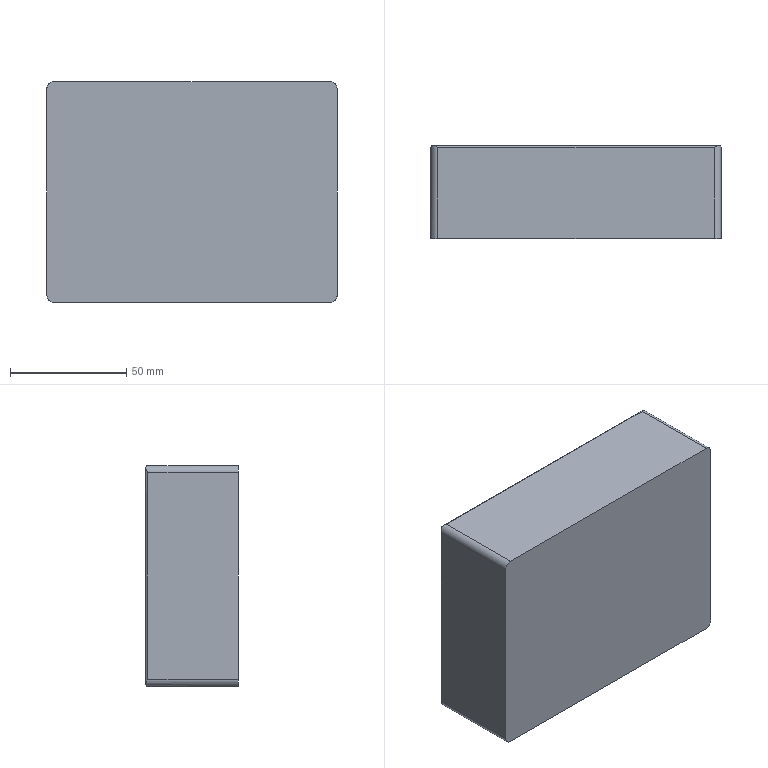Part | SolidWorks | features BaseBody 1 | 1 solid | 20 faces | box 125 x 40 x 95 mm | volume 474597 mm3 | cylinder 8 | cone 6 | plane 6 | commonest cylinder face diameters 2 x4 6 x4
STEP:
#1=CARTESIAN_POINT('',(353.,-93.,-55.087));
#2=VERTEX_POINT('',#1);
#3=CARTESIAN_POINT('',(353.,-92.,-56.087));
#4=VERTEX_POINT('',#3);
#5=CARTESIAN_POINT('',(353.,-92.,-56.087));
#6=DIRECTION('',(0.,0.7071,-0.7071));
#7=VECTOR('',#6,1000.);
#8=LINE('',#5,#7);
#9=EDGE_CURVE('',#2,#4,#8,.T.);
#10=ORIENTED_EDGE('',*,*,#9,.F.);
#11=CARTESIAN_POINT('',(353.,-94.,-56.087));
#12=VERTEX_POINT('',#11);
#13=CARTESIAN_POINT('',(353.,-94.,-56.087));
#14=DIRECTION('',(0.,-0.7071,-0.7071));
#15=VECTOR('',#14,1000.);
#16=LINE('',#13,#15);
#17=EDGE_CURVE('',#2,#12,#16,.T.);
#18=ORIENTED_EDGE('',*,*,#17,.T.);
#19=CARTESIAN_POINT('',(353.,-93.,-56.087));
#20=DIRECTION('',(0.,0.,1.));
#21=DIRECTION('',(0.,1.,0.));
#22=AXIS2_PLACEMENT_3D('',#19,#20,#21);
#23=CIRCLE('',#22,1.);
#24=EDGE_CURVE('',#4,#12,#23,.T.);
#25=ORIENTED_EDGE('',*,*,#24,.F.);
#26=EDGE_LOOP('',(#10,#18,#25));
#27=FACE_OUTER_BOUND('',#26,.T.);
#28=CARTESIAN_POINT('',(353.,-93.,-56.087));
#29=DIRECTION('',(0.,0.,-1.));
#30=DIRECTION('',(0.,1.,0.));
#31=AXIS2_PLACEMENT_3D('',#28,#29,#30);
#32=CONICAL_SURFACE('',#31,1.,0.7854);
#33=ADVANCED_FACE('',(#27),#32,.F.);
#34=CARTESIAN_POINT('',(284.,-93.,-55.087));
#35=VERTEX_POINT('',#34);
#36=CARTESIAN_POINT('',(283.,-93.,-56.087));
#37=VERTEX_POINT('',#36);
#38=CARTESIAN_POINT('',(283.,-93.,-56.087));
#39=DIRECTION('',(-0.7071,0.,-0.7071));
#40=VECTOR('',#39,1000.);
#41=LINE('',#38,#40);
#42=EDGE_CURVE('',#35,#37,#41,.T.);
#43=ORIENTED_EDGE('',*,*,#42,.F.);
#44=CARTESIAN_POINT('',(285.,-93.,-56.087));
#45=VERTEX_POINT('',#44);
#46=CARTESIAN_POINT('',(285.,-93.,-56.087));
#47=DIRECTION('',(0.7071,0.,-0.7071));
#48=VECTOR('',#47,1000.);
#49=LINE('',#46,#48);
#50=EDGE_CURVE('',#35,#45,#49,.T.);
#51=ORIENTED_EDGE('',*,*,#50,.T.);
#52=CARTESIAN_POINT('',(284.,-93.,-56.087));
#53=DIRECTION('',(0.,0.,1.));
#54=DIRECTION('',(-1.,0.,0.));
#55=AXIS2_PLACEMENT_3D('',#52,#53,#54);
#56=CIRCLE('',#55,1.);
#57=EDGE_CURVE('',#37,#45,#56,.T.);
#58=ORIENTED_EDGE('',*,*,#57,.F.);
#59=EDGE_LOOP('',(#43,#51,#58));
#60=FACE_OUTER_BOUND('',#59,.T.);
#61=CARTESIAN_POINT('',(284.,-93.,-56.087));
#62=DIRECTION('',(0.,0.,-1.));
#63=DIRECTION('',(-1.,0.,0.));
#64=AXIS2_PLACEMENT_3D('',#61,#62,#63);
#65=CONICAL_SURFACE('',#64,1.,0.7854);
#66=ADVANCED_FACE('',(#60),#65,.F.);
#67=CARTESIAN_POINT('',(320.,-93.,-55.087));
#68=VERTEX_POINT('',#67);
#69=CARTESIAN_POINT('',(319.,-93.,-56.087));
#70=VERTEX_POINT('',#69);
#71=CARTESIAN_POINT('',(319.,-93.,-56.087));
#72=DIRECTION('',(-0.7071,0.,-0.7071));
#73=VECTOR('',#72,1000.);
#74=LINE('',#71,#73);
#75=EDGE_CURVE('',#68,#70,#74,.T.);
#76=ORIENTED_EDGE('',*,*,#75,.F.);
#77=CARTESIAN_POINT('',(321.,-93.,-56.087));
#78=VERTEX_POINT('',#77);
#79=CARTESIAN_POINT('',(321.,-93.,-56.087));
#80=DIRECTION('',(0.7071,0.,-0.7071));
#81=VECTOR('',#80,1000.);
#82=LINE('',#79,#81);
#83=EDGE_CURVE('',#68,#78,#82,.T.);
#84=ORIENTED_EDGE('',*,*,#83,.T.);
#85=CARTESIAN_POINT('',(320.,-93.,-56.087));
#86=DIRECTION('',(0.,0.,1.));
#87=DIRECTION('',(-1.,0.,0.));
#88=AXIS2_PLACEMENT_3D('',#85,#86,#87);
#89=CIRCLE('',#88,1.);
#90=EDGE_CURVE('',#70,#78,#89,.T.);
#91=ORIENTED_EDGE('',*,*,#90,.F.);
#92=EDGE_LOOP('',(#76,#84,#91));
#93=FACE_OUTER_BOUND('',#92,.T.);
#94=CARTESIAN_POINT('',(320.,-93.,-56.087));
#95=DIRECTION('',(0.,0.,-1.));
#96=DIRECTION('',(-1.,0.,0.));
#97=AXIS2_PLACEMENT_3D('',#94,#95,#96);
#98=CONICAL_SURFACE('',#97,1.,0.7854);
#99=ADVANCED_FACE('',(#93),#98,.F.);
#100=CARTESIAN_POINT('',(381.5,-114.,38.913));
#101=VERTEX_POINT('',#100);
#102=CARTESIAN_POINT('',(262.5,-114.,38.913));
#103=VERTEX_POINT('',#102);
#104=CARTESIAN_POINT('',(322.,-114.,38.913));
#105=DIRECTION('',(-1.,0.,0.));
#106=VECTOR('',#105,1000.);
#107=LINE('',#104,#106);
#108=EDGE_CURVE('',#101,#103,#107,.T.);
#109=ORIENTED_EDGE('',*,*,#108,.T.);
#110=CARTESIAN_POINT('',(259.5,-114.,35.913));
#111=VERTEX_POINT('',#110);
#112=CARTESIAN_POINT('',(262.5,-114.,35.913));
#113=DIRECTION('',(0.,-1.,0.));
#114=DIRECTION('',(0.,0.,-1.));
#115=AXIS2_PLACEMENT_3D('',#112,#113,#114);
#116=CIRCLE('',#115,3.);
#117=EDGE_CURVE('',#103,#111,#116,.T.);
#118=ORIENTED_EDGE('',*,*,#117,.T.);
#119=CARTESIAN_POINT('',(259.5,-114.,-53.087));
#120=VERTEX_POINT('',#119);
#121=CARTESIAN_POINT('',(259.5,-114.,-8.587));
#122=DIRECTION('',(0.,0.,-1.));
#123=VECTOR('',#122,1000.);
#124=LINE('',#121,#123);
#125=EDGE_CURVE('',#111,#120,#124,.T.);
#126=ORIENTED_EDGE('',*,*,#125,.T.);
#127=CARTESIAN_POINT('',(262.5,-114.,-56.087));
#128=VERTEX_POINT('',#127);
#129=CARTESIAN_POINT('',(262.5,-114.,-53.087));
#130=DIRECTION('',(0.,-1.,0.));
#131=DIRECTION('',(0.,0.,-1.));
#132=AXIS2_PLACEMENT_3D('',#129,#130,#131);
#133=CIRCLE('',#132,3.);
#134=EDGE_CURVE('',#120,#128,#133,.T.);
#135=ORIENTED_EDGE('',*,*,#134,.T.);
#136=CARTESIAN_POINT('',(381.5,-114.,-56.087));
#137=VERTEX_POINT('',#136);
#138=CARTESIAN_POINT('',(322.,-114.,-56.087));
#139=DIRECTION('',(1.,0.,0.));
#140=VECTOR('',#139,1000.);
#141=LINE('',#138,#140);
#142=EDGE_CURVE('',#128,#137,#141,.T.);
#143=ORIENTED_EDGE('',*,*,#142,.T.);
#144=CARTESIAN_POINT('',(384.5,-114.,-53.087));
#145=VERTEX_POINT('',#144);
#146=CARTESIAN_POINT('',(381.5,-114.,-53.087));
#147=DIRECTION('',(0.,-1.,0.));
#148=DIRECTION('',(0.,0.,-1.));
#149=AXIS2_PLACEMENT_3D('',#146,#147,#148);
#150=CIRCLE('',#149,3.);
#151=EDGE_CURVE('',#137,#145,#150,.T.);
#152=ORIENTED_EDGE('',*,*,#151,.T.);
#153=CARTESIAN_POINT('',(384.5,-114.,35.913));
#154=VERTEX_POINT('',#153);
#155=CARTESIAN_POINT('',(384.5,-114.,-8.587));
#156=DIRECTION('',(0.,0.,1.));
#157=VECTOR('',#156,1000.);
#158=LINE('',#155,#157);
#159=EDGE_CURVE('',#145,#154,#158,.T.);
#160=ORIENTED_EDGE('',*,*,#159,.T.);
#161=CARTESIAN_POINT('',(381.5,-114.,35.913));
#162=DIRECTION('',(0.,-1.,0.));
#163=DIRECTION('',(0.,0.,-1.));
#164=AXIS2_PLACEMENT_3D('',#161,#162,#163);
#165=CIRCLE('',#164,3.);
#166=EDGE_CURVE('',#154,#101,#165,.T.);
#167=ORIENTED_EDGE('',*,*,#166,.T.);
#168=EDGE_LOOP('',(#109,#118,#126,#135,#143,#152,#160,#167));
#169=FACE_OUTER_BOUND('',#168,.T.);
#170=CARTESIAN_POINT('',(322.,-114.,-8.587));
#171=DIRECTION('',(0.,-1.,0.));
#172=DIRECTION('',(0.,0.,-1.));
#173=AXIS2_PLACEMENT_3D('',#170,#171,#172);
#174=PLANE('',#173);
#175=ADVANCED_FACE('',(#169),#174,.T.);
#176=CARTESIAN_POINT('',(262.5,-75.,38.913));
#177=VERTEX_POINT('',#176);
#178=CARTESIAN_POINT('',(262.5,-74.,38.913));
#179=DIRECTION('',(0.,1.,0.));
#180=VECTOR('',#179,1000.);
#181=LINE('',#178,#180);
#182=EDGE_CURVE('',#103,#177,#181,.T.);
#183=ORIENTED_EDGE('',*,*,#182,.T.);
#184=CARTESIAN_POINT('',(260.379,-74.007,38.034));
#185=VERTEX_POINT('',#184);
#186=CARTESIAN_POINT('',(262.5,-75.,38.913));
#187=CARTESIAN_POINT('',(262.408,-74.947,38.913));
#188=CARTESIAN_POINT('',(262.314,-74.892,38.909));
#189=CARTESIAN_POINT('',(262.129,-74.786,38.891));
#190=CARTESIAN_POINT('',(262.037,-74.734,38.878));
#191=CARTESIAN_POINT('',(261.762,-74.579,38.827));
#192=CARTESIAN_POINT('',(261.58,-74.48,38.775));
#193=CARTESIAN_POINT('',(261.216,-74.295,38.631));
#194=CARTESIAN_POINT('',(261.039,-74.211,38.541));
#195=CARTESIAN_POINT('',(260.697,-74.077,38.319));
#196=CARTESIAN_POINT('',(260.531,-74.026,38.186));
#197=CARTESIAN_POINT('',(260.379,-74.007,38.034));
#198=B_SPLINE_CURVE_WITH_KNOTS('',3,(#186,#187,#188,#189,#190,#191,#192,#193,#194,#195,#196,#197),.UNSPECIFIED.,.F.,.F.,(4,2,2,2,2,4),(-0.00001095,0.0003086,0.0006282,0.001267,0.001907,0.002546),.UNSPECIFIED.);
#199=EDGE_CURVE('',#177,#185,#198,.T.);
#200=ORIENTED_EDGE('',*,*,#199,.T.);
#201=CARTESIAN_POINT('',(259.5,-75.,35.913));
#202=VERTEX_POINT('',#201);
#203=CARTESIAN_POINT('',(260.379,-74.007,38.034));
#204=CARTESIAN_POINT('',(260.226,-74.026,37.881));
#205=CARTESIAN_POINT('',(260.096,-74.076,37.719));
#206=CARTESIAN_POINT('',(259.872,-74.211,37.374));
#207=CARTESIAN_POINT('',(259.782,-74.294,37.198));
#208=CARTESIAN_POINT('',(259.569,-74.568,36.659));
#209=CARTESIAN_POINT('',(259.5,-74.786,36.284));
#210=CARTESIAN_POINT('',(259.5,-75.,35.913));
#211=B_SPLINE_CURVE_WITH_KNOTS('',3,(#203,#204,#205,#206,#207,#208,#209,#210),.UNSPECIFIED.,.F.,.F.,(4,2,2,4),(0.,0.0006423,0.001285,0.002569),.UNSPECIFIED.);
#212=EDGE_CURVE('',#185,#202,#211,.T.);
#213=ORIENTED_EDGE('',*,*,#212,.T.);
#214=CARTESIAN_POINT('',(259.5,-74.,35.913));
#215=DIRECTION('',(0.,-1.,0.));
#216=VECTOR('',#215,1000.);
#217=LINE('',#214,#216);
#218=EDGE_CURVE('',#202,#111,#217,.T.);
#219=ORIENTED_EDGE('',*,*,#218,.T.);
#220=ORIENTED_EDGE('',*,*,#117,.F.);
#221=EDGE_LOOP('',(#183,#200,#213,#219,#220));
#222=FACE_OUTER_BOUND('',#221,.T.);
#223=CARTESIAN_POINT('',(262.5,-74.,35.913));
#224=DIRECTION('',(0.,-1.,0.));
#225=DIRECTION('',(0.,0.,-1.));
#226=AXIS2_PLACEMENT_3D('',#223,#224,#225);
#227=CYLINDRICAL_SURFACE('',#226,3.);
#228=ADVANCED_FACE('',(#222),#227,.T.);
#229=CARTESIAN_POINT('',(381.5,-75.,38.913));
#230=VERTEX_POINT('',#229);
#231=CARTESIAN_POINT('',(262.5,-75.,38.913));
#232=DIRECTION('',(-1.,0.,0.));
#233=VECTOR('',#232,1000.);
#234=LINE('',#231,#233);
#235=EDGE_CURVE('',#230,#177,#234,.T.);
#236=ORIENTED_EDGE('',*,*,#235,.T.);
#237=ORIENTED_EDGE('',*,*,#182,.F.);
#238=ORIENTED_EDGE('',*,*,#108,.F.);
#239=CARTESIAN_POINT('',(381.5,-74.,38.913));
#240=DIRECTION('',(0.,1.,0.));
#241=VECTOR('',#240,1000.);
#242=LINE('',#239,#241);
#243=EDGE_CURVE('',#101,#230,#242,.T.);
#244=ORIENTED_EDGE('',*,*,#243,.T.);
#245=EDGE_LOOP('',(#236,#237,#238,#244));
#246=FACE_OUTER_BOUND('',#245,.T.);
#247=CARTESIAN_POINT('',(262.5,-74.,38.913));
#248=DIRECTION('',(0.,0.,1.));
#249=DIRECTION('',(1.,0.,0.));
#250=AXIS2_PLACEMENT_3D('',#247,#248,#249);
#251=PLANE('',#250);
#252=ADVANCED_FACE('',(#246),#251,.T.);
#253=CARTESIAN_POINT('',(384.5,-75.,35.913));
#254=VERTEX_POINT('',#253);
#255=CARTESIAN_POINT('',(383.621,-74.007,38.034));
#256=VERTEX_POINT('',#255);
#257=CARTESIAN_POINT('',(384.5,-75.,35.913));
#258=CARTESIAN_POINT('',(384.5,-74.947,36.005));
#259=CARTESIAN_POINT('',(384.496,-74.892,36.099));
#260=CARTESIAN_POINT('',(384.478,-74.786,36.284));
#261=CARTESIAN_POINT('',(384.465,-74.734,36.376));
#262=CARTESIAN_POINT('',(384.414,-74.579,36.651));
#263=CARTESIAN_POINT('',(384.362,-74.48,36.833));
#264=CARTESIAN_POINT('',(384.218,-74.295,37.197));
#265=CARTESIAN_POINT('',(384.128,-74.211,37.374));
#266=CARTESIAN_POINT('',(383.906,-74.077,37.716));
#267=CARTESIAN_POINT('',(383.773,-74.026,37.882));
#268=CARTESIAN_POINT('',(383.621,-74.007,38.034));
#269=B_SPLINE_CURVE_WITH_KNOTS('',3,(#257,#258,#259,#260,#261,#262,#263,#264,#265,#266,#267,#268),.UNSPECIFIED.,.F.,.F.,(4,2,2,2,2,4),(-0.00001095,0.0003086,0.0006282,0.001267,0.001907,0.002546),.UNSPECIFIED.);
#270=EDGE_CURVE('',#254,#256,#269,.T.);
#271=ORIENTED_EDGE('',*,*,#270,.T.);
#272=CARTESIAN_POINT('',(383.621,-74.007,38.034));
#273=CARTESIAN_POINT('',(383.468,-74.026,38.187));
#274=CARTESIAN_POINT('',(383.306,-74.076,38.317));
#275=CARTESIAN_POINT('',(382.961,-74.211,38.541));
#276=CARTESIAN_POINT('',(382.785,-74.294,38.631));
#277=CARTESIAN_POINT('',(382.246,-74.568,38.844));
#278=CARTESIAN_POINT('',(381.871,-74.786,38.913));
#279=CARTESIAN_POINT('',(381.5,-75.,38.913));
#280=B_SPLINE_CURVE_WITH_KNOTS('',3,(#272,#273,#274,#275,#276,#277,#278,#279),.UNSPECIFIED.,.F.,.F.,(4,2,2,4),(0.,0.0006423,0.001285,0.002569),.UNSPECIFIED.);
#281=EDGE_CURVE('',#256,#230,#280,.T.);
#282=ORIENTED_EDGE('',*,*,#281,.T.);
#283=ORIENTED_EDGE('',*,*,#243,.F.);
#284=ORIENTED_EDGE('',*,*,#166,.F.);
#285=CARTESIAN_POINT('',(384.5,-74.,35.913));
#286=DIRECTION('',(0.,1.,0.));
#287=VECTOR('',#286,1000.);
#288=LINE('',#285,#287);
#289=EDGE_CURVE('',#154,#254,#288,.T.);
#290=ORIENTED_EDGE('',*,*,#289,.T.);
#291=EDGE_LOOP('',(#271,#282,#283,#284,#290));
#292=FACE_OUTER_BOUND('',#291,.T.);
#293=CARTESIAN_POINT('',(381.5,-74.,35.913));
#294=DIRECTION('',(0.,-1.,0.));
#295=DIRECTION('',(0.,0.,-1.));
#296=AXIS2_PLACEMENT_3D('',#293,#294,#295);
#297=CYLINDRICAL_SURFACE('',#296,3.);
#298=ADVANCED_FACE('',(#292),#297,.T.);
#299=CARTESIAN_POINT('',(384.5,-75.,-53.087));
#300=VERTEX_POINT('',#299);
#301=CARTESIAN_POINT('',(384.5,-75.,35.913));
#302=DIRECTION('',(0.,0.,1.));
#303=VECTOR('',#302,1000.);
#304=LINE('',#301,#303);
#305=EDGE_CURVE('',#300,#254,#304,.T.);
#306=ORIENTED_EDGE('',*,*,#305,.T.);
#307=ORIENTED_EDGE('',*,*,#289,.F.);
#308=ORIENTED_EDGE('',*,*,#159,.F.);
#309=CARTESIAN_POINT('',(384.5,-74.,-53.087));
#310=DIRECTION('',(0.,1.,0.));
#311=VECTOR('',#310,1000.);
#312=LINE('',#309,#311);
#313=EDGE_CURVE('',#145,#300,#312,.T.);
#314=ORIENTED_EDGE('',*,*,#313,.T.);
#315=EDGE_LOOP('',(#306,#307,#308,#314));
#316=FACE_OUTER_BOUND('',#315,.T.);
#317=CARTESIAN_POINT('',(384.5,-74.,35.913));
#318=DIRECTION('',(1.,0.,0.));
#319=DIRECTION('',(0.,0.,-1.));
#320=AXIS2_PLACEMENT_3D('',#317,#318,#319);
#321=PLANE('',#320);
#322=ADVANCED_FACE('',(#316),#321,.T.);
#323=CARTESIAN_POINT('',(381.5,-75.,-56.087));
#324=VERTEX_POINT('',#323);
#325=CARTESIAN_POINT('',(381.5,-74.,-56.087));
#326=DIRECTION('',(0.,1.,0.));
#327=VECTOR('',#326,1000.);
#328=LINE('',#325,#327);
#329=EDGE_CURVE('',#137,#324,#328,.T.);
#330=ORIENTED_EDGE('',*,*,#329,.T.);
#331=CARTESIAN_POINT('',(383.621,-74.007,-55.208));
#332=VERTEX_POINT('',#331);
#333=CARTESIAN_POINT('',(381.5,-75.,-56.087));
#334=CARTESIAN_POINT('',(381.592,-74.947,-56.087));
#335=CARTESIAN_POINT('',(381.686,-74.892,-56.083));
#336=CARTESIAN_POINT('',(381.871,-74.786,-56.065));
#337=CARTESIAN_POINT('',(381.963,-74.734,-56.052));
#338=CARTESIAN_POINT('',(382.238,-74.579,-56.001));
#339=CARTESIAN_POINT('',(382.42,-74.48,-55.949));
#340=CARTESIAN_POINT('',(382.784,-74.295,-55.805));
#341=CARTESIAN_POINT('',(382.961,-74.211,-55.715));
#342=CARTESIAN_POINT('',(383.303,-74.077,-55.493));
#343=CARTESIAN_POINT('',(383.469,-74.026,-55.36));
#344=CARTESIAN_POINT('',(383.621,-74.007,-55.208));
#345=B_SPLINE_CURVE_WITH_KNOTS('',3,(#333,#334,#335,#336,#337,#338,#339,#340,#341,#342,#343,#344),.UNSPECIFIED.,.F.,.F.,(4,2,2,2,2,4),(-0.00001095,0.0003086,0.0006282,0.001267,0.001907,0.002546),.UNSPECIFIED.);
#346=EDGE_CURVE('',#324,#332,#345,.T.);
#347=ORIENTED_EDGE('',*,*,#346,.T.);
#348=CARTESIAN_POINT('',(383.621,-74.007,-55.208));
#349=CARTESIAN_POINT('',(383.774,-74.026,-55.055));
#350=CARTESIAN_POINT('',(383.904,-74.076,-54.893));
#351=CARTESIAN_POINT('',(384.128,-74.211,-54.548));
#352=CARTESIAN_POINT('',(384.218,-74.294,-54.372));
#353=CARTESIAN_POINT('',(384.431,-74.568,-53.833));
#354=CARTESIAN_POINT('',(384.5,-74.786,-53.458));
#355=CARTESIAN_POINT('',(384.5,-75.,-53.087));
#356=B_SPLINE_CURVE_WITH_KNOTS('',3,(#348,#349,#350,#351,#352,#353,#354,#355),.UNSPECIFIED.,.F.,.F.,(4,2,2,4),(0.,0.0006423,0.001285,0.002569),.UNSPECIFIED.);
#357=EDGE_CURVE('',#332,#300,#356,.T.);
#358=ORIENTED_EDGE('',*,*,#357,.T.);
#359=ORIENTED_EDGE('',*,*,#313,.F.);
#360=ORIENTED_EDGE('',*,*,#151,.F.);
#361=EDGE_LOOP('',(#330,#347,#358,#359,#360));
#362=FACE_OUTER_BOUND('',#361,.T.);
#363=CARTESIAN_POINT('',(381.5,-74.,-53.087));
#364=DIRECTION('',(0.,-1.,0.));
#365=DIRECTION('',(0.,0.,-1.));
#366=AXIS2_PLACEMENT_3D('',#363,#364,#365);
#367=CYLINDRICAL_SURFACE('',#366,3.);
#368=ADVANCED_FACE('',(#362),#367,.T.);
#369=ORIENTED_EDGE('',*,*,#24,.T.);
#370=CARTESIAN_POINT('',(353.,-93.,-56.087));
#371=DIRECTION('',(0.,0.,1.));
#372=DIRECTION('',(0.,1.,0.));
#373=AXIS2_PLACEMENT_3D('',#370,#371,#372);
#374=CIRCLE('',#373,1.);
#375=EDGE_CURVE('',#12,#4,#374,.T.);
#376=ORIENTED_EDGE('',*,*,#375,.T.);
#377=EDGE_LOOP('',(#369,#376));
#378=FACE_BOUND('',#377,.T.);
#379=ORIENTED_EDGE('',*,*,#57,.T.);
#380=CARTESIAN_POINT('',(284.,-93.,-56.087));
#381=DIRECTION('',(0.,0.,1.));
#382=DIRECTION('',(-1.,0.,0.));
#383=AXIS2_PLACEMENT_3D('',#380,#381,#382);
#384=CIRCLE('',#383,1.);
#385=EDGE_CURVE('',#45,#37,#384,.T.);
#386=ORIENTED_EDGE('',*,*,#385,.T.);
#387=EDGE_LOOP('',(#379,#386));
#388=FACE_BOUND('',#387,.T.);
#389=ORIENTED_EDGE('',*,*,#90,.T.);
#390=CARTESIAN_POINT('',(320.,-93.,-56.087));
#391=DIRECTION('',(0.,0.,1.));
#392=DIRECTION('',(-1.,0.,0.));
#393=AXIS2_PLACEMENT_3D('',#390,#391,#392);
#394=CIRCLE('',#393,1.);
#395=EDGE_CURVE('',#78,#70,#394,.T.);
#396=ORIENTED_EDGE('',*,*,#395,.T.);
#397=EDGE_LOOP('',(#389,#396));
#398=FACE_BOUND('',#397,.T.);
#399=CARTESIAN_POINT('',(262.5,-75.,-56.087));
#400=VERTEX_POINT('',#399);
#401=CARTESIAN_POINT('',(381.5,-75.,-56.087));
#402=DIRECTION('',(1.,0.,0.));
#403=VECTOR('',#402,1000.);
#404=LINE('',#401,#403);
#405=EDGE_CURVE('',#400,#324,#404,.T.);
#406=ORIENTED_EDGE('',*,*,#405,.T.);
#407=ORIENTED_EDGE('',*,*,#329,.F.);
#408=ORIENTED_EDGE('',*,*,#142,.F.);
#409=CARTESIAN_POINT('',(262.5,-74.,-56.087));
#410=DIRECTION('',(0.,1.,0.));
#411=VECTOR('',#410,1000.);
#412=LINE('',#409,#411);
#413=EDGE_CURVE('',#128,#400,#412,.T.);
#414=ORIENTED_EDGE('',*,*,#413,.T.);
#415=EDGE_LOOP('',(#406,#407,#408,#414));
#416=FACE_OUTER_BOUND('',#415,.T.);
#417=CARTESIAN_POINT('',(381.5,-74.,-56.087));
#418=DIRECTION('',(0.,0.,-1.));
#419=DIRECTION('',(-1.,0.,0.));
#420=AXIS2_PLACEMENT_3D('',#417,#418,#419);
#421=PLANE('',#420);
#422=ADVANCED_FACE('',(#378,#388,#398,#416),#421,.T.);
#423=CARTESIAN_POINT('',(259.5,-75.,-53.087));
#424=VERTEX_POINT('',#423);
#425=CARTESIAN_POINT('',(260.379,-74.007,-55.208));
#426=VERTEX_POINT('',#425);
#427=CARTESIAN_POINT('',(259.5,-75.,-53.087));
#428=CARTESIAN_POINT('',(259.5,-74.947,-53.179));
#429=CARTESIAN_POINT('',(259.504,-74.892,-53.273));
#430=CARTESIAN_POINT('',(259.522,-74.786,-53.458));
#431=CARTESIAN_POINT('',(259.535,-74.734,-53.55));
#432=CARTESIAN_POINT('',(259.586,-74.579,-53.825));
#433=CARTESIAN_POINT('',(259.638,-74.48,-54.007));
#434=CARTESIAN_POINT('',(259.782,-74.295,-54.371));
#435=CARTESIAN_POINT('',(259.872,-74.211,-54.548));
#436=CARTESIAN_POINT('',(260.094,-74.077,-54.89));
#437=CARTESIAN_POINT('',(260.227,-74.026,-55.056));
#438=CARTESIAN_POINT('',(260.379,-74.007,-55.208));
#439=B_SPLINE_CURVE_WITH_KNOTS('',3,(#427,#428,#429,#430,#431,#432,#433,#434,#435,#436,#437,#438),.UNSPECIFIED.,.F.,.F.,(4,2,2,2,2,4),(-0.00001095,0.0003086,0.0006282,0.001267,0.001907,0.002546),.UNSPECIFIED.);
#440=EDGE_CURVE('',#424,#426,#439,.T.);
#441=ORIENTED_EDGE('',*,*,#440,.T.);
#442=CARTESIAN_POINT('',(260.379,-74.007,-55.208));
#443=CARTESIAN_POINT('',(260.532,-74.026,-55.361));
#444=CARTESIAN_POINT('',(260.694,-74.076,-55.491));
#445=CARTESIAN_POINT('',(261.039,-74.211,-55.715));
#446=CARTESIAN_POINT('',(261.215,-74.294,-55.805));
#447=CARTESIAN_POINT('',(261.754,-74.568,-56.018));
#448=CARTESIAN_POINT('',(262.129,-74.786,-56.087));
#449=CARTESIAN_POINT('',(262.5,-75.,-56.087));
#450=B_SPLINE_CURVE_WITH_KNOTS('',3,(#442,#443,#444,#445,#446,#447,#448,#449),.UNSPECIFIED.,.F.,.F.,(4,2,2,4),(0.,0.0006423,0.001285,0.002569),.UNSPECIFIED.);
#451=EDGE_CURVE('',#426,#400,#450,.T.);
#452=ORIENTED_EDGE('',*,*,#451,.T.);
#453=ORIENTED_EDGE('',*,*,#413,.F.);
#454=ORIENTED_EDGE('',*,*,#134,.F.);
#455=CARTESIAN_POINT('',(259.5,-74.,-53.087));
#456=DIRECTION('',(0.,1.,0.));
#457=VECTOR('',#456,1000.);
#458=LINE('',#455,#457);
#459=EDGE_CURVE('',#120,#424,#458,.T.);
#460=ORIENTED_EDGE('',*,*,#459,.T.);
#461=EDGE_LOOP('',(#441,#452,#453,#454,#460));
#462=FACE_OUTER_BOUND('',#461,.T.);
#463=CARTESIAN_POINT('',(262.5,-74.,-53.087));
#464=DIRECTION('',(0.,-1.,0.));
#465=DIRECTION('',(0.,0.,-1.));
#466=AXIS2_PLACEMENT_3D('',#463,#464,#465);
#467=CYLINDRICAL_SURFACE('',#466,3.);
#468=ADVANCED_FACE('',(#462),#467,.T.);
#469=CARTESIAN_POINT('',(259.5,-75.,-10.087));
#470=DIRECTION('',(0.,0.,-1.));
#471=VECTOR('',#470,1000.);
#472=LINE('',#469,#471);
#473=EDGE_CURVE('',#202,#424,#472,.T.);
#474=ORIENTED_EDGE('',*,*,#473,.T.);
#475=ORIENTED_EDGE('',*,*,#459,.F.);
#476=ORIENTED_EDGE('',*,*,#125,.F.);
#477=ORIENTED_EDGE('',*,*,#218,.F.);
#478=EDGE_LOOP('',(#474,#475,#476,#477));
#479=FACE_OUTER_BOUND('',#478,.T.);
#480=CARTESIAN_POINT('',(259.5,-74.,-10.087));
#481=DIRECTION('',(-1.,0.,0.));
#482=DIRECTION('',(0.,0.,1.));
#483=AXIS2_PLACEMENT_3D('',#480,#481,#482);
#484=PLANE('',#483);
#485=ADVANCED_FACE('',(#479),#484,.T.);
#486=ORIENTED_EDGE('',*,*,#235,.F.);
#487=ORIENTED_EDGE('',*,*,#281,.F.);
#488=CARTESIAN_POINT('',(383.5,-74.,37.913));
#489=VERTEX_POINT('',#488);
#490=CARTESIAN_POINT('',(383.621,-74.007,38.034));
#491=CARTESIAN_POINT('',(383.581,-74.002,37.994));
#492=CARTESIAN_POINT('',(383.541,-74.,37.954));
#493=CARTESIAN_POINT('',(383.5,-74.,37.913));
#494=(BOUNDED_CURVE()B_SPLINE_CURVE(3,(#490,#491,#492,#493),.UNSPECIFIED.,.F.,.F.)B_SPLINE_CURVE_WITH_KNOTS((4,4),(4.591,4.712),.UNSPECIFIED.)CURVE()GEOMETRIC_REPRESENTATION_ITEM()RATIONAL_B_SPLINE_CURVE((1.,0.9988,0.9988,1.))REPRESENTATION_ITEM(''));
#495=EDGE_CURVE('',#256,#489,#494,.T.);
#496=ORIENTED_EDGE('',*,*,#495,.T.);
#497=CARTESIAN_POINT('',(260.5,-74.,37.913));
#498=VERTEX_POINT('',#497);
#499=CARTESIAN_POINT('',(384.5,-74.,37.913));
#500=DIRECTION('',(-1.,0.,0.));
#501=VECTOR('',#500,1000.);
#502=LINE('',#499,#501);
#503=EDGE_CURVE('',#489,#498,#502,.T.);
#504=ORIENTED_EDGE('',*,*,#503,.T.);
#505=CARTESIAN_POINT('',(260.5,-74.,37.913));
#506=CARTESIAN_POINT('',(260.459,-74.,37.954));
#507=CARTESIAN_POINT('',(260.419,-74.002,37.994));
#508=CARTESIAN_POINT('',(260.379,-74.007,38.034));
#509=(BOUNDED_CURVE()B_SPLINE_CURVE(3,(#505,#506,#507,#508),.UNSPECIFIED.,.F.,.T.)B_SPLINE_CURVE_WITH_KNOTS((4,4),(4.712,4.834),.UNSPECIFIED.)CURVE()GEOMETRIC_REPRESENTATION_ITEM()RATIONAL_B_SPLINE_CURVE((1.,0.9988,0.9988,1.))REPRESENTATION_ITEM(''));
#510=EDGE_CURVE('',#498,#185,#509,.T.);
#511=ORIENTED_EDGE('',*,*,#510,.T.);
#512=ORIENTED_EDGE('',*,*,#199,.F.);
#513=EDGE_LOOP('',(#486,#487,#496,#504,#511,#512));
#514=FACE_OUTER_BOUND('',#513,.T.);
#515=CARTESIAN_POINT('',(384.5,-75.,37.913));
#516=DIRECTION('',(-1.,0.,0.));
#517=DIRECTION('',(0.,0.,1.));
#518=AXIS2_PLACEMENT_3D('',#515,#516,#517);
#519=CYLINDRICAL_SURFACE('',#518,1.);
#520=ADVANCED_FACE('',(#514),#519,.T.);
#521=CARTESIAN_POINT('',(260.5,-74.,-55.087));
#522=VERTEX_POINT('',#521);
#523=CARTESIAN_POINT('',(260.5,-74.,38.913));
#524=DIRECTION('',(0.,0.,-1.));
#525=VECTOR('',#524,1000.);
#526=LINE('',#523,#525);
#527=EDGE_CURVE('',#498,#522,#526,.T.);
#528=ORIENTED_EDGE('',*,*,#527,.T.);
#529=CARTESIAN_POINT('',(260.5,-74.,-55.087));
#530=CARTESIAN_POINT('',(260.459,-74.,-55.128));
#531=CARTESIAN_POINT('',(260.419,-74.002,-55.168));
#532=CARTESIAN_POINT('',(260.379,-74.007,-55.208));
#533=(BOUNDED_CURVE()B_SPLINE_CURVE(3,(#529,#530,#531,#532),.UNSPECIFIED.,.F.,.T.)B_SPLINE_CURVE_WITH_KNOTS((4,4),(4.712,4.834),.UNSPECIFIED.)CURVE()GEOMETRIC_REPRESENTATION_ITEM()RATIONAL_B_SPLINE_CURVE((1.,0.9988,0.9988,1.))REPRESENTATION_ITEM(''));
#534=EDGE_CURVE('',#522,#426,#533,.T.);
#535=ORIENTED_EDGE('',*,*,#534,.T.);
#536=ORIENTED_EDGE('',*,*,#440,.F.);
#537=ORIENTED_EDGE('',*,*,#473,.F.);
#538=ORIENTED_EDGE('',*,*,#212,.F.);
#539=ORIENTED_EDGE('',*,*,#510,.F.);
#540=EDGE_LOOP('',(#528,#535,#536,#537,#538,#539));
#541=FACE_OUTER_BOUND('',#540,.T.);
#542=CARTESIAN_POINT('',(260.5,-75.,38.913));
#543=DIRECTION('',(0.,0.,-1.));
#544=DIRECTION('',(-1.,0.,0.));
#545=AXIS2_PLACEMENT_3D('',#542,#543,#544);
#546=CYLINDRICAL_SURFACE('',#545,1.);
#547=ADVANCED_FACE('',(#541),#546,.T.);
#548=ORIENTED_EDGE('',*,*,#357,.F.);
#549=CARTESIAN_POINT('',(383.5,-74.,-55.087));
#550=VERTEX_POINT('',#549);
#551=CARTESIAN_POINT('',(383.621,-74.007,-55.208));
#552=CARTESIAN_POINT('',(383.581,-74.002,-55.168));
#553=CARTESIAN_POINT('',(383.541,-74.,-55.128));
#554=CARTESIAN_POINT('',(383.5,-74.,-55.087));
#555=(BOUNDED_CURVE()B_SPLINE_CURVE(3,(#551,#552,#553,#554),.UNSPECIFIED.,.F.,.F.)B_SPLINE_CURVE_WITH_KNOTS((4,4),(1.449,1.571),.UNSPECIFIED.)CURVE()GEOMETRIC_REPRESENTATION_ITEM()RATIONAL_B_SPLINE_CURVE((1.,0.9988,0.9988,1.))REPRESENTATION_ITEM(''));
#556=EDGE_CURVE('',#332,#550,#555,.T.);
#557=ORIENTED_EDGE('',*,*,#556,.T.);
#558=CARTESIAN_POINT('',(383.5,-74.,38.913));
#559=DIRECTION('',(0.,0.,1.));
#560=VECTOR('',#559,1000.);
#561=LINE('',#558,#560);
#562=EDGE_CURVE('',#550,#489,#561,.T.);
#563=ORIENTED_EDGE('',*,*,#562,.T.);
#564=ORIENTED_EDGE('',*,*,#495,.F.);
#565=ORIENTED_EDGE('',*,*,#270,.F.);
#566=ORIENTED_EDGE('',*,*,#305,.F.);
#567=EDGE_LOOP('',(#548,#557,#563,#564,#565,#566));
#568=FACE_OUTER_BOUND('',#567,.T.);
#569=CARTESIAN_POINT('',(383.5,-75.,38.913));
#570=DIRECTION('',(0.,0.,-1.));
#571=DIRECTION('',(-1.,0.,0.));
#572=AXIS2_PLACEMENT_3D('',#569,#570,#571);
#573=CYLINDRICAL_SURFACE('',#572,1.);
#574=ADVANCED_FACE('',(#568),#573,.T.);
#575=ORIENTED_EDGE('',*,*,#556,.F.);
#576=ORIENTED_EDGE('',*,*,#346,.F.);
#577=ORIENTED_EDGE('',*,*,#405,.F.);
#578=ORIENTED_EDGE('',*,*,#451,.F.);
#579=ORIENTED_EDGE('',*,*,#534,.F.);
#580=CARTESIAN_POINT('',(384.5,-74.,-55.087));
#581=DIRECTION('',(1.,0.,0.));
#582=VECTOR('',#581,1000.);
#583=LINE('',#580,#582);
#584=EDGE_CURVE('',#522,#550,#583,.T.);
#585=ORIENTED_EDGE('',*,*,#584,.T.);
#586=EDGE_LOOP('',(#575,#576,#577,#578,#579,#585));
#587=FACE_OUTER_BOUND('',#586,.T.);
#588=CARTESIAN_POINT('',(384.5,-75.,-55.087));
#589=DIRECTION('',(-1.,0.,0.));
#590=DIRECTION('',(0.,0.,1.));
#591=AXIS2_PLACEMENT_3D('',#588,#589,#590);
#592=CYLINDRICAL_SURFACE('',#591,1.);
#593=ADVANCED_FACE('',(#587),#592,.T.);
#594=ORIENTED_EDGE('',*,*,#17,.F.);
#595=ORIENTED_EDGE('',*,*,#9,.T.);
#596=ORIENTED_EDGE('',*,*,#375,.F.);
#597=EDGE_LOOP('',(#594,#595,#596));
#598=FACE_OUTER_BOUND('',#597,.T.);
#599=CARTESIAN_POINT('',(353.,-93.,-56.087));
#600=DIRECTION('',(0.,0.,-1.));
#601=DIRECTION('',(0.,1.,0.));
#602=AXIS2_PLACEMENT_3D('',#599,#600,#601);
#603=CONICAL_SURFACE('',#602,1.,0.7854);
#604=ADVANCED_FACE('',(#598),#603,.F.);
#605=ORIENTED_EDGE('',*,*,#50,.F.);
#606=ORIENTED_EDGE('',*,*,#42,.T.);
#607=ORIENTED_EDGE('',*,*,#385,.F.);
#608=EDGE_LOOP('',(#605,#606,#607));
#609=FACE_OUTER_BOUND('',#608,.T.);
#610=CARTESIAN_POINT('',(284.,-93.,-56.087));
#611=DIRECTION('',(0.,0.,-1.));
#612=DIRECTION('',(-1.,0.,0.));
#613=AXIS2_PLACEMENT_3D('',#610,#611,#612);
#614=CONICAL_SURFACE('',#613,1.,0.7854);
#615=ADVANCED_FACE('',(#609),#614,.F.);
#616=ORIENTED_EDGE('',*,*,#83,.F.);
#617=ORIENTED_EDGE('',*,*,#75,.T.);
#618=ORIENTED_EDGE('',*,*,#395,.F.);
#619=EDGE_LOOP('',(#616,#617,#618));
#620=FACE_OUTER_BOUND('',#619,.T.);
#621=CARTESIAN_POINT('',(320.,-93.,-56.087));
#622=DIRECTION('',(0.,0.,-1.));
#623=DIRECTION('',(-1.,0.,0.));
#624=AXIS2_PLACEMENT_3D('',#621,#622,#623);
#625=CONICAL_SURFACE('',#624,1.,0.7854);
#626=ADVANCED_FACE('',(#620),#625,.F.);
#627=ORIENTED_EDGE('',*,*,#503,.F.);
#628=ORIENTED_EDGE('',*,*,#562,.F.);
#629=ORIENTED_EDGE('',*,*,#584,.F.);
#630=ORIENTED_EDGE('',*,*,#527,.F.);
#631=EDGE_LOOP('',(#627,#628,#629,#630));
#632=FACE_OUTER_BOUND('',#631,.T.);
#633=CARTESIAN_POINT('',(322.,-74.,-8.587));
#634=DIRECTION('',(0.,-1.,0.));
#635=DIRECTION('',(0.,0.,-1.));
#636=AXIS2_PLACEMENT_3D('',#633,#634,#635);
#637=PLANE('',#636);
#638=ADVANCED_FACE('',(#632),#637,.F.);
#639=CLOSED_SHELL('',(#33,#66,#99,#175,#228,#252,#298,#322,#368,#422,#468,#485,#520,#547,#574,#593,#604,#615,#626,#638));
#640=MANIFOLD_SOLID_BREP('',#639);
#641=CARTESIAN_POINT('',(0.,0.,0.));
#642=DIRECTION('',(0.,0.,1.));
#643=DIRECTION('',(1.,0.,0.));
#644=AXIS2_PLACEMENT_3D('',#641,#642,#643);
#645=(LENGTH_UNIT()NAMED_UNIT(*)SI_UNIT(.MILLI.,.METRE.));
#646=UNCERTAINTY_MEASURE_WITH_UNIT(LENGTH_MEASURE(0.00001),#645,'','');
#647=(NAMED_UNIT(*)PLANE_ANGLE_UNIT()SI_UNIT($,.RADIAN.));
#648=(NAMED_UNIT(*)SI_UNIT($,.STERADIAN.)SOLID_ANGLE_UNIT());
#649=(GEOMETRIC_REPRESENTATION_CONTEXT(3)GLOBAL_UNCERTAINTY_ASSIGNED_CONTEXT((#646))GLOBAL_UNIT_ASSIGNED_CONTEXT((#645,#647,#648))REPRESENTATION_CONTEXT('',''));
#650=ADVANCED_BREP_SHAPE_REPRESENTATION('',(#640,#644),#649);